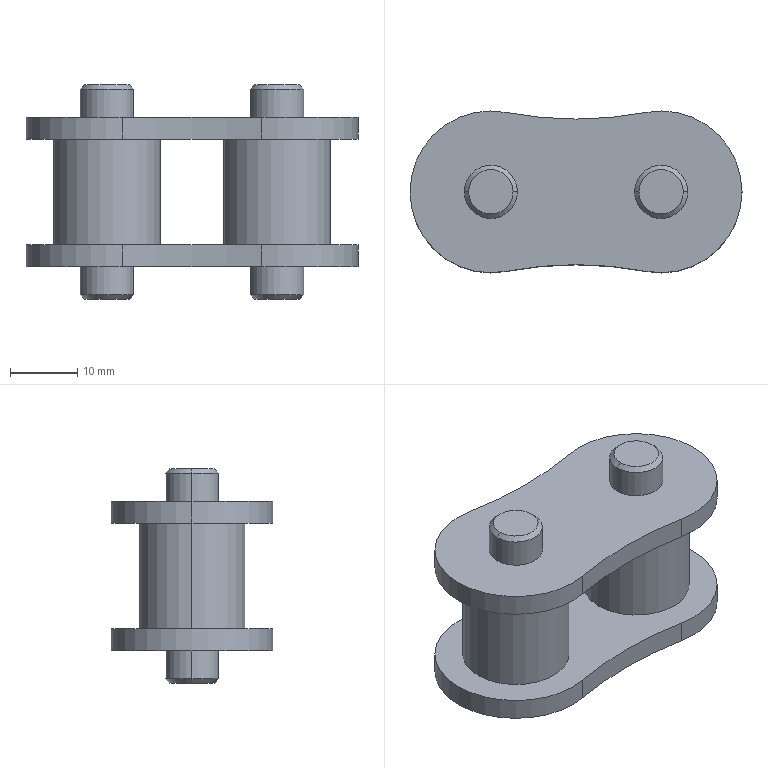Part | STEP file | Inner chain link | 1 solid | 38 faces | box 49.53 x 24.13 x 32 mm | volume 13899 mm3 | cylinder 22 | cone 8 | plane 8 | commonest cylinder face diameters 7.94 x8 24.13 x6 15.88 x4 110.761 x4